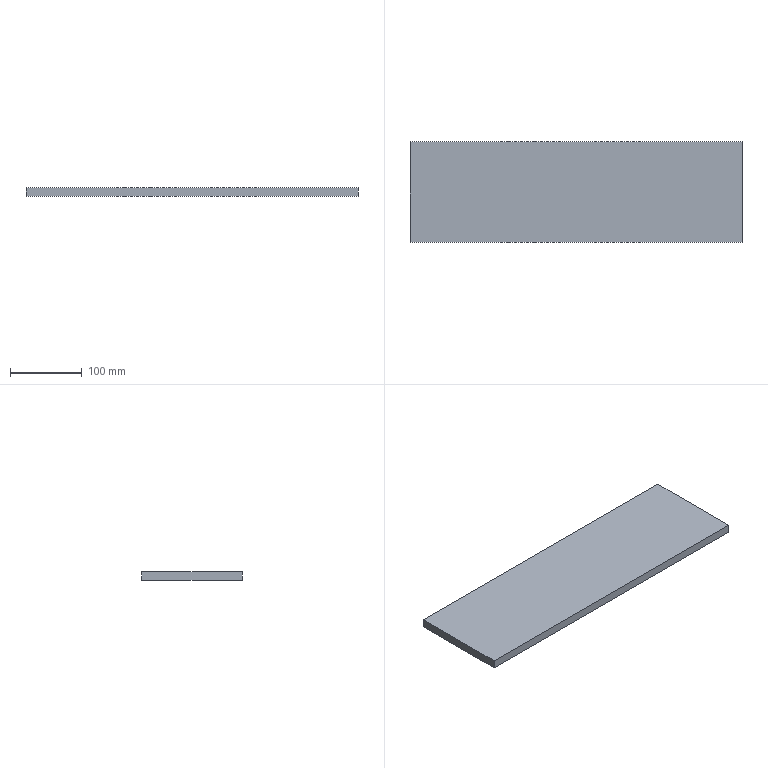Part | STEP file | Upper and lower bearing mounting plate | 1 solid | 6 faces | box 463 x 140 x 12 mm | volume 777840 mm3 | plane 6
STEP:
#1=CARTESIAN_POINT('',(231.5,-70.,0.));
#2=VERTEX_POINT('',#1);
#3=CARTESIAN_POINT('',(231.5,70.,0.));
#4=VERTEX_POINT('',#3);
#5=CARTESIAN_POINT('',(231.5,-70.,0.));
#6=DIRECTION('',(0.,1.,0.));
#7=VECTOR('',#6,1000.);
#8=LINE('',#5,#7);
#9=EDGE_CURVE('',#2,#4,#8,.T.);
#10=ORIENTED_EDGE('',*,*,#9,.T.);
#11=CARTESIAN_POINT('',(231.5,70.,12.));
#12=VERTEX_POINT('',#11);
#13=CARTESIAN_POINT('',(231.5,70.,12.));
#14=DIRECTION('',(0.,0.,-1.));
#15=VECTOR('',#14,1000.);
#16=LINE('',#13,#15);
#17=EDGE_CURVE('',#12,#4,#16,.T.);
#18=ORIENTED_EDGE('',*,*,#17,.F.);
#19=CARTESIAN_POINT('',(231.5,-70.,12.));
#20=VERTEX_POINT('',#19);
#21=CARTESIAN_POINT('',(231.5,-70.,12.));
#22=DIRECTION('',(0.,1.,0.));
#23=VECTOR('',#22,1000.);
#24=LINE('',#21,#23);
#25=EDGE_CURVE('',#20,#12,#24,.T.);
#26=ORIENTED_EDGE('',*,*,#25,.F.);
#27=CARTESIAN_POINT('',(231.5,-70.,12.));
#28=DIRECTION('',(0.,0.,-1.));
#29=VECTOR('',#28,1000.);
#30=LINE('',#27,#29);
#31=EDGE_CURVE('',#20,#2,#30,.T.);
#32=ORIENTED_EDGE('',*,*,#31,.T.);
#33=EDGE_LOOP('',(#10,#18,#26,#32));
#34=FACE_OUTER_BOUND('',#33,.T.);
#35=CARTESIAN_POINT('',(231.5,-70.,12.));
#36=DIRECTION('',(-1.,0.,0.));
#37=DIRECTION('',(0.,0.,1.));
#38=AXIS2_PLACEMENT_3D('',#35,#36,#37);
#39=PLANE('',#38);
#40=ADVANCED_FACE('',(#34),#39,.F.);
#41=CARTESIAN_POINT('',(-231.5,70.,0.));
#42=VERTEX_POINT('',#41);
#43=CARTESIAN_POINT('',(-231.5,70.,0.));
#44=DIRECTION('',(-1.,0.,0.));
#45=VECTOR('',#44,1000.);
#46=LINE('',#43,#45);
#47=EDGE_CURVE('',#4,#42,#46,.T.);
#48=ORIENTED_EDGE('',*,*,#47,.T.);
#49=CARTESIAN_POINT('',(-231.5,70.,12.));
#50=VERTEX_POINT('',#49);
#51=CARTESIAN_POINT('',(-231.5,70.,12.));
#52=DIRECTION('',(0.,0.,-1.));
#53=VECTOR('',#52,1000.);
#54=LINE('',#51,#53);
#55=EDGE_CURVE('',#50,#42,#54,.T.);
#56=ORIENTED_EDGE('',*,*,#55,.F.);
#57=CARTESIAN_POINT('',(-231.5,70.,12.));
#58=DIRECTION('',(-1.,0.,0.));
#59=VECTOR('',#58,1000.);
#60=LINE('',#57,#59);
#61=EDGE_CURVE('',#12,#50,#60,.T.);
#62=ORIENTED_EDGE('',*,*,#61,.F.);
#63=ORIENTED_EDGE('',*,*,#17,.T.);
#64=EDGE_LOOP('',(#48,#56,#62,#63));
#65=FACE_OUTER_BOUND('',#64,.T.);
#66=CARTESIAN_POINT('',(-231.5,70.,12.));
#67=DIRECTION('',(0.,-1.,0.));
#68=DIRECTION('',(0.,0.,-1.));
#69=AXIS2_PLACEMENT_3D('',#66,#67,#68);
#70=PLANE('',#69);
#71=ADVANCED_FACE('',(#65),#70,.F.);
#72=CARTESIAN_POINT('',(-231.5,-70.,0.));
#73=VERTEX_POINT('',#72);
#74=CARTESIAN_POINT('',(-231.5,-70.,0.));
#75=DIRECTION('',(0.,-1.,0.));
#76=VECTOR('',#75,1000.);
#77=LINE('',#74,#76);
#78=EDGE_CURVE('',#42,#73,#77,.T.);
#79=ORIENTED_EDGE('',*,*,#78,.T.);
#80=CARTESIAN_POINT('',(-231.5,-70.,12.));
#81=VERTEX_POINT('',#80);
#82=CARTESIAN_POINT('',(-231.5,-70.,12.));
#83=DIRECTION('',(0.,0.,-1.));
#84=VECTOR('',#83,1000.);
#85=LINE('',#82,#84);
#86=EDGE_CURVE('',#81,#73,#85,.T.);
#87=ORIENTED_EDGE('',*,*,#86,.F.);
#88=CARTESIAN_POINT('',(-231.5,-70.,12.));
#89=DIRECTION('',(0.,-1.,0.));
#90=VECTOR('',#89,1000.);
#91=LINE('',#88,#90);
#92=EDGE_CURVE('',#50,#81,#91,.T.);
#93=ORIENTED_EDGE('',*,*,#92,.F.);
#94=ORIENTED_EDGE('',*,*,#55,.T.);
#95=EDGE_LOOP('',(#79,#87,#93,#94));
#96=FACE_OUTER_BOUND('',#95,.T.);
#97=CARTESIAN_POINT('',(-231.5,-70.,12.));
#98=DIRECTION('',(1.,0.,0.));
#99=DIRECTION('',(0.,0.,-1.));
#100=AXIS2_PLACEMENT_3D('',#97,#98,#99);
#101=PLANE('',#100);
#102=ADVANCED_FACE('',(#96),#101,.F.);
#103=CARTESIAN_POINT('',(-231.5,-70.,0.));
#104=DIRECTION('',(1.,0.,0.));
#105=VECTOR('',#104,1000.);
#106=LINE('',#103,#105);
#107=EDGE_CURVE('',#73,#2,#106,.T.);
#108=ORIENTED_EDGE('',*,*,#107,.T.);
#109=ORIENTED_EDGE('',*,*,#31,.F.);
#110=CARTESIAN_POINT('',(-231.5,-70.,12.));
#111=DIRECTION('',(1.,0.,0.));
#112=VECTOR('',#111,1000.);
#113=LINE('',#110,#112);
#114=EDGE_CURVE('',#81,#20,#113,.T.);
#115=ORIENTED_EDGE('',*,*,#114,.F.);
#116=ORIENTED_EDGE('',*,*,#86,.T.);
#117=EDGE_LOOP('',(#108,#109,#115,#116));
#118=FACE_OUTER_BOUND('',#117,.T.);
#119=CARTESIAN_POINT('',(-231.5,-70.,12.));
#120=DIRECTION('',(0.,1.,0.));
#121=DIRECTION('',(0.,0.,1.));
#122=AXIS2_PLACEMENT_3D('',#119,#120,#121);
#123=PLANE('',#122);
#124=ADVANCED_FACE('',(#118),#123,.F.);
#125=ORIENTED_EDGE('',*,*,#25,.T.);
#126=ORIENTED_EDGE('',*,*,#61,.T.);
#127=ORIENTED_EDGE('',*,*,#92,.T.);
#128=ORIENTED_EDGE('',*,*,#114,.T.);
#129=EDGE_LOOP('',(#125,#126,#127,#128));
#130=FACE_OUTER_BOUND('',#129,.T.);
#131=CARTESIAN_POINT('',(0.,0.,12.));
#132=DIRECTION('',(0.,0.,-1.));
#133=DIRECTION('',(-1.,0.,0.));
#134=AXIS2_PLACEMENT_3D('',#131,#132,#133);
#135=PLANE('',#134);
#136=ADVANCED_FACE('',(#130),#135,.F.);
#137=ORIENTED_EDGE('',*,*,#9,.F.);
#138=ORIENTED_EDGE('',*,*,#107,.F.);
#139=ORIENTED_EDGE('',*,*,#78,.F.);
#140=ORIENTED_EDGE('',*,*,#47,.F.);
#141=EDGE_LOOP('',(#137,#138,#139,#140));
#142=FACE_OUTER_BOUND('',#141,.T.);
#143=CARTESIAN_POINT('',(0.,0.,0.));
#144=DIRECTION('',(0.,0.,-1.));
#145=DIRECTION('',(-1.,0.,0.));
#146=AXIS2_PLACEMENT_3D('',#143,#144,#145);
#147=PLANE('',#146);
#148=ADVANCED_FACE('',(#142),#147,.T.);
#149=CLOSED_SHELL('',(#40,#71,#102,#124,#136,#148));
#150=MANIFOLD_SOLID_BREP('',#149);
#151=CARTESIAN_POINT('',(0.,0.,0.));
#152=DIRECTION('',(0.,0.,1.));
#153=DIRECTION('',(1.,0.,0.));
#154=AXIS2_PLACEMENT_3D('',#151,#152,#153);
#155=(LENGTH_UNIT()NAMED_UNIT(*)SI_UNIT(.MILLI.,.METRE.));
#156=UNCERTAINTY_MEASURE_WITH_UNIT(LENGTH_MEASURE(0.00001),#155,'','');
#157=(NAMED_UNIT(*)PLANE_ANGLE_UNIT()SI_UNIT($,.RADIAN.));
#158=(NAMED_UNIT(*)SI_UNIT($,.STERADIAN.)SOLID_ANGLE_UNIT());
#159=(GEOMETRIC_REPRESENTATION_CONTEXT(3)GLOBAL_UNCERTAINTY_ASSIGNED_CONTEXT((#156))GLOBAL_UNIT_ASSIGNED_CONTEXT((#155,#157,#158))REPRESENTATION_CONTEXT('',''));
#160=ADVANCED_BREP_SHAPE_REPRESENTATION('',(#150,#154),#159);